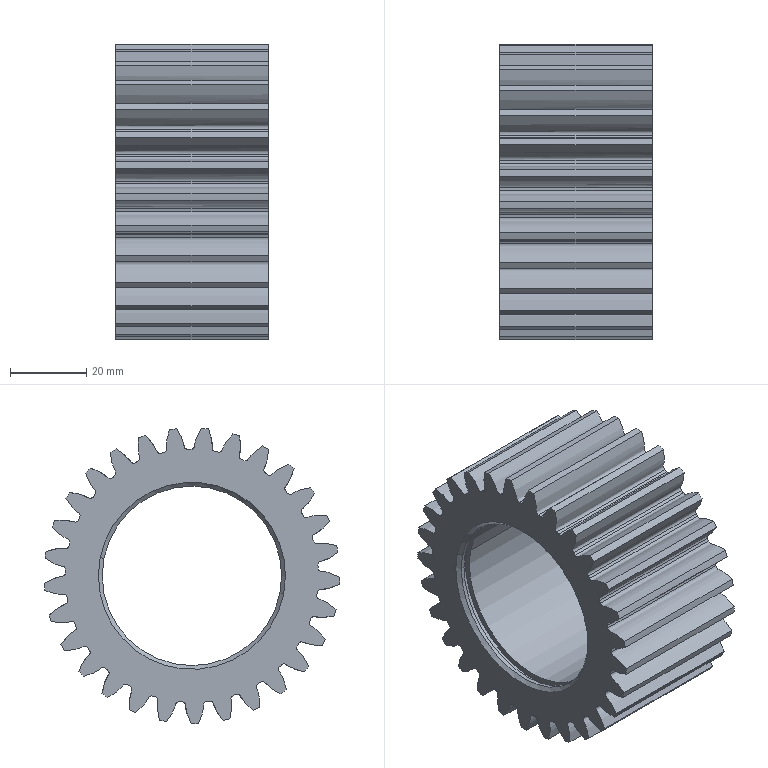Part | NX | features BREP 1 | 1 solid | 136 faces | box 40 x 77.448 x 77.419 mm | volume 92521 mm3 | cylinder 68 | spline 58 | plane 6 | cone 4 | commonest cylinder face diameters 66.25 x29 77.5 x29 47 x6 50 x4